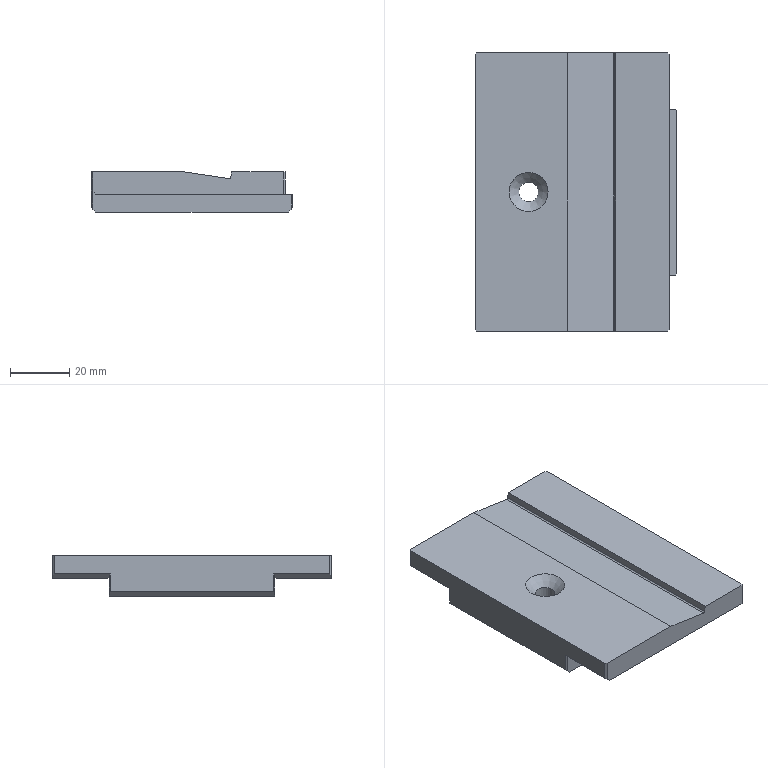Part | NX | 1 solid | 30 faces | box 68 x 94 x 13.65 mm | volume 67246 mm3 | plane 27 | cylinder 2 | cone 1 | commonest cylinder face diameters 1 x1 6.6 x1
STEP:
#1=CARTESIAN_POINT('',(-34.,27.5,1.5));
#2=VERTEX_POINT('',#1);
#3=CARTESIAN_POINT('',(-34.,-27.5,1.5));
#4=VERTEX_POINT('',#3);
#5=CARTESIAN_POINT('',(-34.,47.,1.5));
#6=DIRECTION('',(0.,-1.,0.));
#7=VECTOR('',#6,1000.);
#8=LINE('',#5,#7);
#9=EDGE_CURVE('',#2,#4,#8,.T.);
#10=ORIENTED_EDGE('',*,*,#9,.T.);
#11=CARTESIAN_POINT('',(-34.,-27.5,7.5));
#12=VERTEX_POINT('',#11);
#13=CARTESIAN_POINT('',(-34.,-27.5,13.65));
#14=DIRECTION('',(0.,0.,1.));
#15=VECTOR('',#14,1000.);
#16=LINE('',#13,#15);
#17=EDGE_CURVE('',#4,#12,#16,.T.);
#18=ORIENTED_EDGE('',*,*,#17,.T.);
#19=CARTESIAN_POINT('',(-34.,-46.5,7.5));
#20=VERTEX_POINT('',#19);
#21=CARTESIAN_POINT('',(-34.,47.,7.5));
#22=DIRECTION('',(0.,1.,0.));
#23=VECTOR('',#22,1000.);
#24=LINE('',#21,#23);
#25=EDGE_CURVE('',#12,#20,#24,.F.);
#26=ORIENTED_EDGE('',*,*,#25,.T.);
#27=CARTESIAN_POINT('',(-34.,-46.5,13.65));
#28=VERTEX_POINT('',#27);
#29=CARTESIAN_POINT('',(-34.,-46.5,13.65));
#30=DIRECTION('',(0.,0.,1.));
#31=VECTOR('',#30,1000.);
#32=LINE('',#29,#31);
#33=EDGE_CURVE('',#20,#28,#32,.T.);
#34=ORIENTED_EDGE('',*,*,#33,.T.);
#35=CARTESIAN_POINT('',(-34.,46.5,13.65));
#36=VERTEX_POINT('',#35);
#37=CARTESIAN_POINT('',(-34.,47.,13.65));
#38=DIRECTION('',(0.,-1.,0.));
#39=VECTOR('',#38,1000.);
#40=LINE('',#37,#39);
#41=EDGE_CURVE('',#36,#28,#40,.T.);
#42=ORIENTED_EDGE('',*,*,#41,.F.);
#43=CARTESIAN_POINT('',(-34.,46.5,7.5));
#44=VERTEX_POINT('',#43);
#45=CARTESIAN_POINT('',(-34.,46.5,13.65));
#46=DIRECTION('',(0.,0.,-1.));
#47=VECTOR('',#46,1000.);
#48=LINE('',#45,#47);
#49=EDGE_CURVE('',#36,#44,#48,.T.);
#50=ORIENTED_EDGE('',*,*,#49,.T.);
#51=CARTESIAN_POINT('',(-34.,27.5,7.5));
#52=VERTEX_POINT('',#51);
#53=CARTESIAN_POINT('',(-34.,47.,7.5));
#54=DIRECTION('',(0.,1.,0.));
#55=VECTOR('',#54,1000.);
#56=LINE('',#53,#55);
#57=EDGE_CURVE('',#44,#52,#56,.F.);
#58=ORIENTED_EDGE('',*,*,#57,.T.);
#59=CARTESIAN_POINT('',(-34.,27.5,1.5));
#60=DIRECTION('',(0.,0.,-1.));
#61=VECTOR('',#60,1000.);
#62=LINE('',#59,#61);
#63=EDGE_CURVE('',#52,#2,#62,.T.);
#64=ORIENTED_EDGE('',*,*,#63,.T.);
#65=EDGE_LOOP('',(#10,#18,#26,#34,#42,#50,#58,#64));
#66=FACE_BOUND('',#65,.T.);
#67=CARTESIAN_POINT('',(-34.,47.,13.65));
#68=DIRECTION('',(1.,0.,0.));
#69=DIRECTION('',(0.,0.,-1.));
#70=AXIS2_PLACEMENT_3D('',#67,#68,#69);
#71=PLANE('',#70);
#72=ADVANCED_FACE('',(#66),#71,.F.);
#73=ORIENTED_EDGE('',*,*,#41,.T.);
#74=CARTESIAN_POINT('',(-33.5,-47.,13.65));
#75=VERTEX_POINT('',#74);
#76=CARTESIAN_POINT('',(-48.25,-32.25,13.65));
#77=DIRECTION('',(-0.7071,0.7071,0.));
#78=VECTOR('',#77,1000.);
#79=LINE('',#76,#78);
#80=EDGE_CURVE('',#28,#75,#79,.F.);
#81=ORIENTED_EDGE('',*,*,#80,.T.);
#82=CARTESIAN_POINT('',(-3.,-47.,13.65));
#83=VERTEX_POINT('',#82);
#84=CARTESIAN_POINT('',(-34.,-47.,13.65));
#85=DIRECTION('',(1.,0.,0.));
#86=VECTOR('',#85,1000.);
#87=LINE('',#84,#86);
#88=EDGE_CURVE('',#75,#83,#87,.T.);
#89=ORIENTED_EDGE('',*,*,#88,.T.);
#90=CARTESIAN_POINT('',(-3.,47.,13.65));
#91=VERTEX_POINT('',#90);
#92=CARTESIAN_POINT('',(-3.,0.,13.65));
#93=DIRECTION('',(0.,1.,0.));
#94=VECTOR('',#93,1000.);
#95=LINE('',#92,#94);
#96=EDGE_CURVE('',#83,#91,#95,.T.);
#97=ORIENTED_EDGE('',*,*,#96,.T.);
#98=CARTESIAN_POINT('',(-33.5,47.,13.65));
#99=VERTEX_POINT('',#98);
#100=CARTESIAN_POINT('',(34.,47.,13.65));
#101=DIRECTION('',(-1.,0.,0.));
#102=VECTOR('',#101,1000.);
#103=LINE('',#100,#102);
#104=EDGE_CURVE('',#91,#99,#103,.T.);
#105=ORIENTED_EDGE('',*,*,#104,.T.);
#106=CARTESIAN_POINT('',(-48.25,32.25,13.65));
#107=DIRECTION('',(0.7071,0.7071,0.));
#108=VECTOR('',#107,1000.);
#109=LINE('',#106,#108);
#110=EDGE_CURVE('',#99,#36,#109,.F.);
#111=ORIENTED_EDGE('',*,*,#110,.T.);
#112=EDGE_LOOP('',(#73,#81,#89,#97,#105,#111));
#113=FACE_BOUND('',#112,.T.);
#114=CARTESIAN_POINT('',(-9.4,0.,13.65));
#115=VERTEX_POINT('',#114);
#116=CARTESIAN_POINT('',(-16.,0.,13.65));
#117=DIRECTION('',(0.,0.,1.));
#118=DIRECTION('',(1.,0.,0.));
#119=AXIS2_PLACEMENT_3D('',#116,#117,#118);
#120=CIRCLE('',#119,6.6);
#121=EDGE_CURVE('',#115,#115,#120,.F.);
#122=ORIENTED_EDGE('',*,*,#121,.T.);
#123=EDGE_LOOP('',(#122));
#124=FACE_BOUND('',#123,.T.);
#125=CARTESIAN_POINT('',(-16.,0.,13.65));
#126=DIRECTION('',(0.,0.,1.));
#127=DIRECTION('',(1.,0.,0.));
#128=AXIS2_PLACEMENT_3D('',#125,#126,#127);
#129=PLANE('',#128);
#130=ADVANCED_FACE('',(#113,#124),#129,.T.);
#131=CARTESIAN_POINT('',(-12.7,0.,0.));
#132=VERTEX_POINT('',#131);
#133=CARTESIAN_POINT('',(-16.,0.,0.));
#134=DIRECTION('',(0.,0.,1.));
#135=DIRECTION('',(1.,0.,0.));
#136=AXIS2_PLACEMENT_3D('',#133,#134,#135);
#137=CIRCLE('',#136,3.3);
#138=EDGE_CURVE('',#132,#132,#137,.T.);
#139=ORIENTED_EDGE('',*,*,#138,.T.);
#140=EDGE_LOOP('',(#139));
#141=FACE_BOUND('',#140,.T.);
#142=CARTESIAN_POINT('',(-32.5,28.,0.));
#143=VERTEX_POINT('',#142);
#144=CARTESIAN_POINT('',(32.5,28.,0.));
#145=VERTEX_POINT('',#144);
#146=CARTESIAN_POINT('',(-16.,28.,0.));
#147=DIRECTION('',(-1.,0.,0.));
#148=VECTOR('',#147,1000.);
#149=LINE('',#146,#148);
#150=EDGE_CURVE('',#143,#145,#149,.F.);
#151=ORIENTED_EDGE('',*,*,#150,.T.);
#152=CARTESIAN_POINT('',(32.5,-28.,0.));
#153=VERTEX_POINT('',#152);
#154=CARTESIAN_POINT('',(32.5,0.,0.));
#155=DIRECTION('',(0.,-1.,0.));
#156=VECTOR('',#155,1000.);
#157=LINE('',#154,#156);
#158=EDGE_CURVE('',#145,#153,#157,.T.);
#159=ORIENTED_EDGE('',*,*,#158,.T.);
#160=CARTESIAN_POINT('',(-32.5,-28.,0.));
#161=VERTEX_POINT('',#160);
#162=CARTESIAN_POINT('',(-16.,-28.,0.));
#163=DIRECTION('',(-1.,0.,0.));
#164=VECTOR('',#163,1000.);
#165=LINE('',#162,#164);
#166=EDGE_CURVE('',#161,#153,#165,.F.);
#167=ORIENTED_EDGE('',*,*,#166,.F.);
#168=CARTESIAN_POINT('',(-32.5,0.,0.));
#169=DIRECTION('',(0.,1.,0.));
#170=VECTOR('',#169,1000.);
#171=LINE('',#168,#170);
#172=EDGE_CURVE('',#161,#143,#171,.T.);
#173=ORIENTED_EDGE('',*,*,#172,.T.);
#174=EDGE_LOOP('',(#151,#159,#167,#173));
#175=FACE_BOUND('',#174,.T.);
#176=CARTESIAN_POINT('',(-16.,0.,0.));
#177=DIRECTION('',(0.,0.,1.));
#178=DIRECTION('',(1.,0.,0.));
#179=AXIS2_PLACEMENT_3D('',#176,#177,#178);
#180=PLANE('',#179);
#181=ADVANCED_FACE('',(#141,#175),#180,.F.);
#182=CARTESIAN_POINT('',(31.4,46.5,13.65));
#183=VERTEX_POINT('',#182);
#184=CARTESIAN_POINT('',(31.4,-46.5,13.65));
#185=VERTEX_POINT('',#184);
#186=CARTESIAN_POINT('',(31.4,0.,13.65));
#187=DIRECTION('',(0.,-1.,0.));
#188=VECTOR('',#187,1000.);
#189=LINE('',#186,#188);
#190=EDGE_CURVE('',#183,#185,#189,.T.);
#191=ORIENTED_EDGE('',*,*,#190,.T.);
#192=CARTESIAN_POINT('',(31.4,-46.5,6.));
#193=VERTEX_POINT('',#192);
#194=CARTESIAN_POINT('',(31.4,-46.5,6.));
#195=DIRECTION('',(0.,0.,-1.));
#196=VECTOR('',#195,1000.);
#197=LINE('',#194,#196);
#198=EDGE_CURVE('',#185,#193,#197,.T.);
#199=ORIENTED_EDGE('',*,*,#198,.T.);
#200=CARTESIAN_POINT('',(31.4,-28.,6.));
#201=VERTEX_POINT('',#200);
#202=CARTESIAN_POINT('',(31.4,0.,6.));
#203=DIRECTION('',(0.,1.,0.));
#204=VECTOR('',#203,1000.);
#205=LINE('',#202,#204);
#206=EDGE_CURVE('',#201,#193,#205,.F.);
#207=ORIENTED_EDGE('',*,*,#206,.F.);
#208=CARTESIAN_POINT('',(31.4,28.,6.));
#209=VERTEX_POINT('',#208);
#210=CARTESIAN_POINT('',(31.4,0.,6.));
#211=DIRECTION('',(0.,1.,0.));
#212=VECTOR('',#211,1000.);
#213=LINE('',#210,#212);
#214=EDGE_CURVE('',#209,#201,#213,.F.);
#215=ORIENTED_EDGE('',*,*,#214,.F.);
#216=CARTESIAN_POINT('',(31.4,46.5,6.));
#217=VERTEX_POINT('',#216);
#218=CARTESIAN_POINT('',(31.4,0.,6.));
#219=DIRECTION('',(0.,1.,0.));
#220=VECTOR('',#219,1000.);
#221=LINE('',#218,#220);
#222=EDGE_CURVE('',#217,#209,#221,.F.);
#223=ORIENTED_EDGE('',*,*,#222,.F.);
#224=CARTESIAN_POINT('',(31.4,46.5,13.65));
#225=DIRECTION('',(0.,0.,1.));
#226=VECTOR('',#225,1000.);
#227=LINE('',#224,#226);
#228=EDGE_CURVE('',#217,#183,#227,.T.);
#229=ORIENTED_EDGE('',*,*,#228,.T.);
#230=EDGE_LOOP('',(#191,#199,#207,#215,#223,#229));
#231=FACE_BOUND('',#230,.T.);
#232=CARTESIAN_POINT('',(31.4,0.,6.825));
#233=DIRECTION('',(1.,0.,0.));
#234=DIRECTION('',(0.,0.,-1.));
#235=AXIS2_PLACEMENT_3D('',#232,#233,#234);
#236=PLANE('',#235);
#237=ADVANCED_FACE('',(#231),#236,.T.);
#238=CARTESIAN_POINT('',(34.,27.5,6.));
#239=VERTEX_POINT('',#238);
#240=CARTESIAN_POINT('',(34.,-27.5,6.));
#241=VERTEX_POINT('',#240);
#242=CARTESIAN_POINT('',(34.,-47.,6.));
#243=DIRECTION('',(0.,-1.,0.));
#244=VECTOR('',#243,1000.);
#245=LINE('',#242,#244);
#246=EDGE_CURVE('',#239,#241,#245,.T.);
#247=ORIENTED_EDGE('',*,*,#246,.T.);
#248=CARTESIAN_POINT('',(34.,-27.5,1.5));
#249=VERTEX_POINT('',#248);
#250=CARTESIAN_POINT('',(34.,-27.5,13.65));
#251=DIRECTION('',(0.,0.,-1.));
#252=VECTOR('',#251,1000.);
#253=LINE('',#250,#252);
#254=EDGE_CURVE('',#241,#249,#253,.T.);
#255=ORIENTED_EDGE('',*,*,#254,.T.);
#256=CARTESIAN_POINT('',(34.,27.5,1.5));
#257=VERTEX_POINT('',#256);
#258=CARTESIAN_POINT('',(34.,-47.,1.5));
#259=DIRECTION('',(0.,1.,0.));
#260=VECTOR('',#259,1000.);
#261=LINE('',#258,#260);
#262=EDGE_CURVE('',#249,#257,#261,.T.);
#263=ORIENTED_EDGE('',*,*,#262,.T.);
#264=CARTESIAN_POINT('',(34.,27.5,6.));
#265=DIRECTION('',(0.,0.,1.));
#266=VECTOR('',#265,1000.);
#267=LINE('',#264,#266);
#268=EDGE_CURVE('',#257,#239,#267,.T.);
#269=ORIENTED_EDGE('',*,*,#268,.T.);
#270=EDGE_LOOP('',(#247,#255,#263,#269));
#271=FACE_BOUND('',#270,.T.);
#272=CARTESIAN_POINT('',(34.,-47.,13.65));
#273=DIRECTION('',(-1.,0.,0.));
#274=DIRECTION('',(0.,0.,1.));
#275=AXIS2_PLACEMENT_3D('',#272,#273,#274);
#276=PLANE('',#275);
#277=ADVANCED_FACE('',(#271),#276,.F.);
#278=CARTESIAN_POINT('',(33.5,-28.,6.));
#279=VERTEX_POINT('',#278);
#280=CARTESIAN_POINT('',(32.7,-28.,6.));
#281=DIRECTION('',(1.,0.,0.));
#282=VECTOR('',#281,1000.);
#283=LINE('',#280,#282);
#284=EDGE_CURVE('',#201,#279,#283,.T.);
#285=ORIENTED_EDGE('',*,*,#284,.T.);
#286=CARTESIAN_POINT('',(33.5,-28.,6.));
#287=DIRECTION('',(-0.7071,-0.7071,0.));
#288=VECTOR('',#287,1000.);
#289=LINE('',#286,#288);
#290=EDGE_CURVE('',#279,#241,#289,.F.);
#291=ORIENTED_EDGE('',*,*,#290,.T.);
#292=ORIENTED_EDGE('',*,*,#246,.F.);
#293=CARTESIAN_POINT('',(33.5,28.,6.));
#294=VERTEX_POINT('',#293);
#295=CARTESIAN_POINT('',(34.,27.5,6.));
#296=DIRECTION('',(-0.7071,0.7071,0.));
#297=VECTOR('',#296,1000.);
#298=LINE('',#295,#297);
#299=EDGE_CURVE('',#239,#294,#298,.T.);
#300=ORIENTED_EDGE('',*,*,#299,.T.);
#301=CARTESIAN_POINT('',(32.7,28.,6.));
#302=DIRECTION('',(1.,0.,0.));
#303=VECTOR('',#302,1000.);
#304=LINE('',#301,#303);
#305=EDGE_CURVE('',#209,#294,#304,.T.);
#306=ORIENTED_EDGE('',*,*,#305,.F.);
#307=ORIENTED_EDGE('',*,*,#214,.T.);
#308=EDGE_LOOP('',(#285,#291,#292,#300,#306,#307));
#309=FACE_BOUND('',#308,.T.);
#310=CARTESIAN_POINT('',(32.7,0.,6.));
#311=DIRECTION('',(0.,0.,-1.));
#312=DIRECTION('',(-1.,0.,0.));
#313=AXIS2_PLACEMENT_3D('',#310,#311,#312);
#314=PLANE('',#313);
#315=ADVANCED_FACE('',(#309),#314,.F.);
#316=ORIENTED_EDGE('',*,*,#96,.F.);
#317=CARTESIAN_POINT('',(12.531,-47.,11.329));
#318=VERTEX_POINT('',#317);
#319=CARTESIAN_POINT('',(-3.,-47.,13.65));
#320=DIRECTION('',(0.989,0.,-0.1478));
#321=VECTOR('',#320,1000.);
#322=LINE('',#319,#321);
#323=EDGE_CURVE('',#83,#318,#322,.T.);
#324=ORIENTED_EDGE('',*,*,#323,.T.);
#325=CARTESIAN_POINT('',(12.531,47.,11.329));
#326=VERTEX_POINT('',#325);
#327=CARTESIAN_POINT('',(12.531,47.,11.329));
#328=DIRECTION('',(0.,-1.,0.));
#329=VECTOR('',#328,1000.);
#330=LINE('',#327,#329);
#331=EDGE_CURVE('',#318,#326,#330,.F.);
#332=ORIENTED_EDGE('',*,*,#331,.T.);
#333=CARTESIAN_POINT('',(-3.,47.,13.65));
#334=DIRECTION('',(0.989,0.,-0.1478));
#335=VECTOR('',#334,1000.);
#336=LINE('',#333,#335);
#337=EDGE_CURVE('',#91,#326,#336,.T.);
#338=ORIENTED_EDGE('',*,*,#337,.F.);
#339=EDGE_LOOP('',(#316,#324,#332,#338));
#340=FACE_BOUND('',#339,.T.);
#341=CARTESIAN_POINT('',(-3.,47.,13.65));
#342=DIRECTION('',(-0.1478,0.,-0.989));
#343=DIRECTION('',(-0.989,0.,0.1478));
#344=AXIS2_PLACEMENT_3D('',#341,#342,#343);
#345=PLANE('',#344);
#346=ADVANCED_FACE('',(#340),#345,.F.);
#347=CARTESIAN_POINT('',(13.099,47.,11.75));
#348=VERTEX_POINT('',#347);
#349=CARTESIAN_POINT('',(13.099,-47.,11.75));
#350=VERTEX_POINT('',#349);
#351=CARTESIAN_POINT('',(13.099,0.,11.75));
#352=DIRECTION('',(0.,-1.,0.));
#353=VECTOR('',#352,1000.);
#354=LINE('',#351,#353);
#355=EDGE_CURVE('',#348,#350,#354,.T.);
#356=ORIENTED_EDGE('',*,*,#355,.T.);
#357=CARTESIAN_POINT('',(13.383,-47.,13.65));
#358=VERTEX_POINT('',#357);
#359=CARTESIAN_POINT('',(13.025,-47.,11.255));
#360=DIRECTION('',(-0.1478,0.,-0.989));
#361=VECTOR('',#360,1000.);
#362=LINE('',#359,#361);
#363=EDGE_CURVE('',#358,#350,#362,.T.);
#364=ORIENTED_EDGE('',*,*,#363,.F.);
#365=CARTESIAN_POINT('',(13.383,47.,13.65));
#366=VERTEX_POINT('',#365);
#367=CARTESIAN_POINT('',(13.383,0.,13.65));
#368=DIRECTION('',(0.,1.,0.));
#369=VECTOR('',#368,1000.);
#370=LINE('',#367,#369);
#371=EDGE_CURVE('',#358,#366,#370,.T.);
#372=ORIENTED_EDGE('',*,*,#371,.T.);
#373=CARTESIAN_POINT('',(13.834,47.,16.664));
#374=DIRECTION('',(-0.1478,0.,-0.989));
#375=VECTOR('',#374,1000.);
#376=LINE('',#373,#375);
#377=EDGE_CURVE('',#366,#348,#376,.T.);
#378=ORIENTED_EDGE('',*,*,#377,.T.);
#379=EDGE_LOOP('',(#356,#364,#372,#378));
#380=FACE_BOUND('',#379,.T.);
#381=CARTESIAN_POINT('',(13.025,0.,11.255));
#382=DIRECTION('',(-0.989,0.,0.1478));
#383=DIRECTION('',(0.1478,0.,0.989));
#384=AXIS2_PLACEMENT_3D('',#381,#382,#383);
#385=PLANE('',#384);
#386=ADVANCED_FACE('',(#380),#385,.T.);
#387=CARTESIAN_POINT('',(30.9,-47.,13.65));
#388=VERTEX_POINT('',#387);
#389=CARTESIAN_POINT('',(-34.,-47.,13.65));
#390=DIRECTION('',(-1.,0.,0.));
#391=VECTOR('',#390,1000.);
#392=LINE('',#389,#391);
#393=EDGE_CURVE('',#388,#358,#392,.T.);
#394=ORIENTED_EDGE('',*,*,#393,.F.);
#395=CARTESIAN_POINT('',(31.4,-46.5,13.65));
#396=DIRECTION('',(0.7071,0.7071,0.));
#397=VECTOR('',#396,1000.);
#398=LINE('',#395,#397);
#399=EDGE_CURVE('',#388,#185,#398,.T.);
#400=ORIENTED_EDGE('',*,*,#399,.T.);
#401=ORIENTED_EDGE('',*,*,#190,.F.);
#402=CARTESIAN_POINT('',(30.9,47.,13.65));
#403=VERTEX_POINT('',#402);
#404=CARTESIAN_POINT('',(31.4,46.5,13.65));
#405=DIRECTION('',(-0.7071,0.7071,0.));
#406=VECTOR('',#405,1000.);
#407=LINE('',#404,#406);
#408=EDGE_CURVE('',#183,#403,#407,.T.);
#409=ORIENTED_EDGE('',*,*,#408,.T.);
#410=CARTESIAN_POINT('',(34.,47.,13.65));
#411=DIRECTION('',(1.,0.,0.));
#412=VECTOR('',#411,1000.);
#413=LINE('',#410,#412);
#414=EDGE_CURVE('',#366,#403,#413,.T.);
#415=ORIENTED_EDGE('',*,*,#414,.F.);
#416=ORIENTED_EDGE('',*,*,#371,.F.);
#417=EDGE_LOOP('',(#394,#400,#401,#409,#415,#416));
#418=FACE_BOUND('',#417,.T.);
#419=CARTESIAN_POINT('',(0.,0.,13.65));
#420=DIRECTION('',(0.,0.,-1.));
#421=DIRECTION('',(-1.,0.,0.));
#422=AXIS2_PLACEMENT_3D('',#419,#420,#421);
#423=PLANE('',#422);
#424=ADVANCED_FACE('',(#418),#423,.F.);
#425=CARTESIAN_POINT('',(-33.5,-28.,1.));
#426=VERTEX_POINT('',#425);
#427=CARTESIAN_POINT('',(-34.,-28.,1.5));
#428=DIRECTION('',(-0.7071,0.,0.7071));
#429=VECTOR('',#428,1000.);
#430=LINE('',#427,#429);
#431=EDGE_CURVE('',#426,#161,#430,.F.);
#432=ORIENTED_EDGE('',*,*,#431,.F.);
#433=CARTESIAN_POINT('',(-58.833,-2.667,26.333));
#434=DIRECTION('',(-0.5774,0.5774,0.5774));
#435=VECTOR('',#434,1000.);
#436=LINE('',#433,#435);
#437=EDGE_CURVE('',#426,#4,#436,.T.);
#438=ORIENTED_EDGE('',*,*,#437,.T.);
#439=ORIENTED_EDGE('',*,*,#9,.F.);
#440=CARTESIAN_POINT('',(-33.5,28.,1.));
#441=VERTEX_POINT('',#440);
#442=CARTESIAN_POINT('',(-27.5,34.,-5.));
#443=DIRECTION('',(-0.5774,-0.5774,0.5774));
#444=VECTOR('',#443,1000.);
#445=LINE('',#442,#444);
#446=EDGE_CURVE('',#2,#441,#445,.F.);
#447=ORIENTED_EDGE('',*,*,#446,.T.);
#448=CARTESIAN_POINT('',(-34.,28.,1.5));
#449=DIRECTION('',(-0.7071,0.,0.7071));
#450=VECTOR('',#449,1000.);
#451=LINE('',#448,#450);
#452=EDGE_CURVE('',#143,#441,#451,.T.);
#453=ORIENTED_EDGE('',*,*,#452,.F.);
#454=ORIENTED_EDGE('',*,*,#172,.F.);
#455=EDGE_LOOP('',(#432,#438,#439,#447,#453,#454));
#456=FACE_BOUND('',#455,.T.);
#457=CARTESIAN_POINT('',(-34.,47.,1.5));
#458=DIRECTION('',(0.7071,0.,0.7071));
#459=DIRECTION('',(0.,-1.,0.));
#460=AXIS2_PLACEMENT_3D('',#457,#458,#459);
#461=PLANE('',#460);
#462=ADVANCED_FACE('',(#456),#461,.F.);
#463=ORIENTED_EDGE('',*,*,#331,.F.);
#464=CARTESIAN_POINT('',(12.605,-47.,11.823));
#465=DIRECTION('',(0.,1.,0.));
#466=DIRECTION('',(0.,0.,1.));
#467=AXIS2_PLACEMENT_3D('',#464,#465,#466);
#468=CIRCLE('',#467,0.5);
#469=EDGE_CURVE('',#350,#318,#468,.T.);
#470=ORIENTED_EDGE('',*,*,#469,.F.);
#471=ORIENTED_EDGE('',*,*,#355,.F.);
#472=CARTESIAN_POINT('',(12.605,47.,11.823));
#473=DIRECTION('',(0.,-1.,0.));
#474=DIRECTION('',(0.,0.,-1.));
#475=AXIS2_PLACEMENT_3D('',#472,#473,#474);
#476=CIRCLE('',#475,0.5);
#477=EDGE_CURVE('',#326,#348,#476,.T.);
#478=ORIENTED_EDGE('',*,*,#477,.F.);
#479=EDGE_LOOP('',(#463,#470,#471,#478));
#480=FACE_BOUND('',#479,.T.);
#481=CARTESIAN_POINT('',(12.605,0.,11.823));
#482=DIRECTION('',(0.,-1.,0.));
#483=DIRECTION('',(0.,0.,-1.));
#484=AXIS2_PLACEMENT_3D('',#481,#482,#483);
#485=CYLINDRICAL_SURFACE('',#484,0.5);
#486=ADVANCED_FACE('',(#480),#485,.F.);
#487=ORIENTED_EDGE('',*,*,#121,.F.);
#488=EDGE_LOOP('',(#487));
#489=FACE_BOUND('',#488,.T.);
#490=CARTESIAN_POINT('',(-12.7,0.,10.35));
#491=VERTEX_POINT('',#490);
#492=CARTESIAN_POINT('',(-16.,0.,10.35));
#493=DIRECTION('',(0.,0.,1.));
#494=DIRECTION('',(1.,0.,0.));
#495=AXIS2_PLACEMENT_3D('',#492,#493,#494);
#496=CIRCLE('',#495,3.3);
#497=EDGE_CURVE('',#491,#491,#496,.T.);
#498=ORIENTED_EDGE('',*,*,#497,.F.);
#499=EDGE_LOOP('',(#498));
#500=FACE_BOUND('',#499,.T.);
#501=CARTESIAN_POINT('',(-16.,0.,10.35));
#502=DIRECTION('',(0.,0.,1.));
#503=DIRECTION('',(1.,0.,0.));
#504=AXIS2_PLACEMENT_3D('',#501,#502,#503);
#505=CONICAL_SURFACE('',#504,3.3,0.7854);
#506=ADVANCED_FACE('',(#489,#500),#505,.F.);
#507=ORIENTED_EDGE('',*,*,#497,.T.);
#508=EDGE_LOOP('',(#507));
#509=FACE_BOUND('',#508,.T.);
#510=ORIENTED_EDGE('',*,*,#138,.F.);
#511=EDGE_LOOP('',(#510));
#512=FACE_BOUND('',#511,.T.);
#513=CARTESIAN_POINT('',(-16.,0.,13.65));
#514=DIRECTION('',(0.,0.,-1.));
#515=DIRECTION('',(-1.,0.,0.));
#516=AXIS2_PLACEMENT_3D('',#513,#514,#515);
#517=CYLINDRICAL_SURFACE('',#516,3.3);
#518=ADVANCED_FACE('',(#509,#512),#517,.F.);
#519=ORIENTED_EDGE('',*,*,#305,.T.);
#520=CARTESIAN_POINT('',(33.5,28.,1.));
#521=VERTEX_POINT('',#520);
#522=CARTESIAN_POINT('',(33.5,28.,1.5));
#523=DIRECTION('',(0.,0.,-1.));
#524=VECTOR('',#523,1000.);
#525=LINE('',#522,#524);
#526=EDGE_CURVE('',#294,#521,#525,.T.);
#527=ORIENTED_EDGE('',*,*,#526,.T.);
#528=CARTESIAN_POINT('',(19.663,28.,-12.838));
#529=DIRECTION('',(0.7071,0.,0.7071));
#530=VECTOR('',#529,1000.);
#531=LINE('',#528,#530);
#532=EDGE_CURVE('',#521,#145,#531,.F.);
#533=ORIENTED_EDGE('',*,*,#532,.T.);
#534=ORIENTED_EDGE('',*,*,#150,.F.);
#535=ORIENTED_EDGE('',*,*,#452,.T.);
#536=CARTESIAN_POINT('',(-33.5,28.,7.));
#537=VERTEX_POINT('',#536);
#538=CARTESIAN_POINT('',(-33.5,28.,7.5));
#539=DIRECTION('',(0.,0.,1.));
#540=VECTOR('',#539,1000.);
#541=LINE('',#538,#540);
#542=EDGE_CURVE('',#441,#537,#541,.T.);
#543=ORIENTED_EDGE('',*,*,#542,.T.);
#544=CARTESIAN_POINT('',(-32.5,28.,6.));
#545=VERTEX_POINT('',#544);
#546=CARTESIAN_POINT('',(-34.,28.,7.5));
#547=DIRECTION('',(-0.7071,0.,0.7071));
#548=VECTOR('',#547,1000.);
#549=LINE('',#546,#548);
#550=EDGE_CURVE('',#537,#545,#549,.F.);
#551=ORIENTED_EDGE('',*,*,#550,.T.);
#552=CARTESIAN_POINT('',(-16.,28.,6.));
#553=DIRECTION('',(-1.,0.,0.));
#554=VECTOR('',#553,1000.);
#555=LINE('',#552,#554);
#556=EDGE_CURVE('',#209,#545,#555,.T.);
#557=ORIENTED_EDGE('',*,*,#556,.F.);
#558=EDGE_LOOP('',(#519,#527,#533,#534,#535,#543,#551,#557));
#559=FACE_BOUND('',#558,.T.);
#560=CARTESIAN_POINT('',(0.,28.,6.825));
#561=DIRECTION('',(0.,1.,0.));
#562=DIRECTION('',(0.,0.,1.));
#563=AXIS2_PLACEMENT_3D('',#560,#561,#562);
#564=PLANE('',#563);
#565=ADVANCED_FACE('',(#559),#564,.T.);
#566=CARTESIAN_POINT('',(33.5,-28.,1.));
#567=VERTEX_POINT('',#566);
#568=CARTESIAN_POINT('',(34.,-28.,1.5));
#569=DIRECTION('',(-0.7071,0.,-0.7071));
#570=VECTOR('',#569,1000.);
#571=LINE('',#568,#570);
#572=EDGE_CURVE('',#153,#567,#571,.F.);
#573=ORIENTED_EDGE('',*,*,#572,.T.);
#574=CARTESIAN_POINT('',(33.5,-28.,6.825));
#575=DIRECTION('',(0.,0.,1.));
#576=VECTOR('',#575,1000.);
#577=LINE('',#574,#576);
#578=EDGE_CURVE('',#567,#279,#577,.T.);
#579=ORIENTED_EDGE('',*,*,#578,.T.);
#580=ORIENTED_EDGE('',*,*,#284,.F.);
#581=CARTESIAN_POINT('',(-32.5,-28.,6.));
#582=VERTEX_POINT('',#581);
#583=CARTESIAN_POINT('',(-16.,-28.,6.));
#584=DIRECTION('',(-1.,0.,0.));
#585=VECTOR('',#584,1000.);
#586=LINE('',#583,#585);
#587=EDGE_CURVE('',#201,#582,#586,.T.);
#588=ORIENTED_EDGE('',*,*,#587,.T.);
#589=CARTESIAN_POINT('',(-33.5,-28.,7.));
#590=VERTEX_POINT('',#589);
#591=CARTESIAN_POINT('',(-16.663,-28.,-9.838));
#592=DIRECTION('',(0.7071,0.,-0.7071));
#593=VECTOR('',#592,1000.);
#594=LINE('',#591,#593);
#595=EDGE_CURVE('',#582,#590,#594,.F.);
#596=ORIENTED_EDGE('',*,*,#595,.T.);
#597=CARTESIAN_POINT('',(-33.5,-28.,6.825));
#598=DIRECTION('',(0.,0.,-1.));
#599=VECTOR('',#598,1000.);
#600=LINE('',#597,#599);
#601=EDGE_CURVE('',#590,#426,#600,.T.);
#602=ORIENTED_EDGE('',*,*,#601,.T.);
#603=ORIENTED_EDGE('',*,*,#431,.T.);
#604=ORIENTED_EDGE('',*,*,#166,.T.);
#605=EDGE_LOOP('',(#573,#579,#580,#588,#596,#602,#603,#604));
#606=FACE_BOUND('',#605,.T.);
#607=CARTESIAN_POINT('',(0.,-28.,6.825));
#608=DIRECTION('',(0.,1.,0.));
#609=DIRECTION('',(0.,0.,1.));
#610=AXIS2_PLACEMENT_3D('',#607,#608,#609);
#611=PLANE('',#610);
#612=ADVANCED_FACE('',(#606),#611,.F.);
#613=ORIENTED_EDGE('',*,*,#414,.T.);
#614=CARTESIAN_POINT('',(30.9,47.,6.));
#615=VERTEX_POINT('',#614);
#616=CARTESIAN_POINT('',(30.9,47.,6.));
#617=DIRECTION('',(0.,0.,-1.));
#618=VECTOR('',#617,1000.);
#619=LINE('',#616,#618);
#620=EDGE_CURVE('',#403,#615,#619,.T.);
#621=ORIENTED_EDGE('',*,*,#620,.T.);
#622=CARTESIAN_POINT('',(-32.5,47.,6.));
#623=VERTEX_POINT('',#622);
#624=CARTESIAN_POINT('',(34.,47.,6.));
#625=DIRECTION('',(-1.,0.,0.));
#626=VECTOR('',#625,1000.);
#627=LINE('',#624,#626);
#628=EDGE_CURVE('',#615,#623,#627,.T.);
#629=ORIENTED_EDGE('',*,*,#628,.T.);
#630=CARTESIAN_POINT('',(-33.5,47.,7.));
#631=VERTEX_POINT('',#630);
#632=CARTESIAN_POINT('',(-34.,47.,7.5));
#633=DIRECTION('',(0.7071,0.,-0.7071));
#634=VECTOR('',#633,1000.);
#635=LINE('',#632,#634);
#636=EDGE_CURVE('',#623,#631,#635,.F.);
#637=ORIENTED_EDGE('',*,*,#636,.T.);
#638=CARTESIAN_POINT('',(-33.5,47.,13.65));
#639=DIRECTION('',(0.,0.,1.));
#640=VECTOR('',#639,1000.);
#641=LINE('',#638,#640);
#642=EDGE_CURVE('',#631,#99,#641,.T.);
#643=ORIENTED_EDGE('',*,*,#642,.T.);
#644=ORIENTED_EDGE('',*,*,#104,.F.);
#645=ORIENTED_EDGE('',*,*,#337,.T.);
#646=ORIENTED_EDGE('',*,*,#477,.T.);
#647=ORIENTED_EDGE('',*,*,#377,.F.);
#648=EDGE_LOOP('',(#613,#621,#629,#637,#643,#644,#645,#646,#647));
#649=FACE_BOUND('',#648,.T.);
#650=CARTESIAN_POINT('',(34.,47.,13.65));
#651=DIRECTION('',(0.,-1.,0.));
#652=DIRECTION('',(0.,0.,-1.));
#653=AXIS2_PLACEMENT_3D('',#650,#651,#652);
#654=PLANE('',#653);
#655=ADVANCED_FACE('',(#649),#654,.F.);
#656=ORIENTED_EDGE('',*,*,#57,.F.);
#657=CARTESIAN_POINT('',(-33.833,46.667,7.333));
#658=DIRECTION('',(0.5774,0.5774,-0.5774));
#659=VECTOR('',#658,1000.);
#660=LINE('',#657,#659);
#661=EDGE_CURVE('',#44,#631,#660,.T.);
#662=ORIENTED_EDGE('',*,*,#661,.T.);
#663=ORIENTED_EDGE('',*,*,#636,.F.);
#664=CARTESIAN_POINT('',(-32.5,47.,6.));
#665=DIRECTION('',(0.,-1.,0.));
#666=VECTOR('',#665,1000.);
#667=LINE('',#664,#666);
#668=EDGE_CURVE('',#545,#623,#667,.F.);
#669=ORIENTED_EDGE('',*,*,#668,.F.);
#670=ORIENTED_EDGE('',*,*,#550,.F.);
#671=CARTESIAN_POINT('',(-36.05,25.45,9.55));
#672=DIRECTION('',(0.5774,0.5774,-0.5774));
#673=VECTOR('',#672,1000.);
#674=LINE('',#671,#673);
#675=EDGE_CURVE('',#537,#52,#674,.F.);
#676=ORIENTED_EDGE('',*,*,#675,.T.);
#677=EDGE_LOOP('',(#656,#662,#663,#669,#670,#676));
#678=FACE_BOUND('',#677,.T.);
#679=CARTESIAN_POINT('',(-34.,47.,7.5));
#680=DIRECTION('',(0.7071,0.,0.7071));
#681=DIRECTION('',(0.7071,0.,-0.7071));
#682=AXIS2_PLACEMENT_3D('',#679,#680,#681);
#683=PLANE('',#682);
#684=ADVANCED_FACE('',(#678),#683,.F.);
#685=ORIENTED_EDGE('',*,*,#628,.F.);
#686=CARTESIAN_POINT('',(31.4,46.5,6.));
#687=DIRECTION('',(0.7071,-0.7071,0.));
#688=VECTOR('',#687,1000.);
#689=LINE('',#686,#688);
#690=EDGE_CURVE('',#615,#217,#689,.T.);
#691=ORIENTED_EDGE('',*,*,#690,.T.);
#692=ORIENTED_EDGE('',*,*,#222,.T.);
#693=ORIENTED_EDGE('',*,*,#556,.T.);
#694=ORIENTED_EDGE('',*,*,#668,.T.);
#695=EDGE_LOOP('',(#685,#691,#692,#693,#694));
#696=FACE_BOUND('',#695,.T.);
#697=CARTESIAN_POINT('',(-16.,0.,6.));
#698=DIRECTION('',(0.,0.,1.));
#699=DIRECTION('',(1.,0.,0.));
#700=AXIS2_PLACEMENT_3D('',#697,#698,#699);
#701=PLANE('',#700);
#702=ADVANCED_FACE('',(#696),#701,.F.);
#703=ORIENTED_EDGE('',*,*,#88,.F.);
#704=CARTESIAN_POINT('',(-33.5,-47.,7.));
#705=VERTEX_POINT('',#704);
#706=CARTESIAN_POINT('',(-33.5,-47.,13.65));
#707=DIRECTION('',(0.,0.,-1.));
#708=VECTOR('',#707,1000.);
#709=LINE('',#706,#708);
#710=EDGE_CURVE('',#75,#705,#709,.T.);
#711=ORIENTED_EDGE('',*,*,#710,.T.);
#712=CARTESIAN_POINT('',(-32.5,-47.,6.));
#713=VERTEX_POINT('',#712);
#714=CARTESIAN_POINT('',(-34.,-47.,7.5));
#715=DIRECTION('',(-0.7071,0.,0.7071));
#716=VECTOR('',#715,1000.);
#717=LINE('',#714,#716);
#718=EDGE_CURVE('',#705,#713,#717,.F.);
#719=ORIENTED_EDGE('',*,*,#718,.T.);
#720=CARTESIAN_POINT('',(30.9,-47.,6.));
#721=VERTEX_POINT('',#720);
#722=CARTESIAN_POINT('',(-34.,-47.,6.));
#723=DIRECTION('',(1.,0.,0.));
#724=VECTOR('',#723,1000.);
#725=LINE('',#722,#724);
#726=EDGE_CURVE('',#713,#721,#725,.T.);
#727=ORIENTED_EDGE('',*,*,#726,.T.);
#728=CARTESIAN_POINT('',(30.9,-47.,13.65));
#729=DIRECTION('',(0.,0.,1.));
#730=VECTOR('',#729,1000.);
#731=LINE('',#728,#730);
#732=EDGE_CURVE('',#721,#388,#731,.T.);
#733=ORIENTED_EDGE('',*,*,#732,.T.);
#734=ORIENTED_EDGE('',*,*,#393,.T.);
#735=ORIENTED_EDGE('',*,*,#363,.T.);
#736=ORIENTED_EDGE('',*,*,#469,.T.);
#737=ORIENTED_EDGE('',*,*,#323,.F.);
#738=EDGE_LOOP('',(#703,#711,#719,#727,#733,#734,#735,#736,#737));
#739=FACE_BOUND('',#738,.T.);
#740=CARTESIAN_POINT('',(-34.,-47.,13.65));
#741=DIRECTION('',(0.,1.,0.));
#742=DIRECTION('',(0.,0.,1.));
#743=AXIS2_PLACEMENT_3D('',#740,#741,#742);
#744=PLANE('',#743);
#745=ADVANCED_FACE('',(#739),#744,.F.);
#746=ORIENTED_EDGE('',*,*,#718,.F.);
#747=CARTESIAN_POINT('',(-65.167,-15.333,38.667));
#748=DIRECTION('',(-0.5774,0.5774,0.5774));
#749=VECTOR('',#748,1000.);
#750=LINE('',#747,#749);
#751=EDGE_CURVE('',#705,#20,#750,.T.);
#752=ORIENTED_EDGE('',*,*,#751,.T.);
#753=ORIENTED_EDGE('',*,*,#25,.F.);
#754=CARTESIAN_POINT('',(-33.442,-28.058,6.942));
#755=DIRECTION('',(0.5774,-0.5774,-0.5774));
#756=VECTOR('',#755,1000.);
#757=LINE('',#754,#756);
#758=EDGE_CURVE('',#12,#590,#757,.T.);
#759=ORIENTED_EDGE('',*,*,#758,.T.);
#760=ORIENTED_EDGE('',*,*,#595,.F.);
#761=CARTESIAN_POINT('',(-32.5,47.,6.));
#762=DIRECTION('',(0.,-1.,0.));
#763=VECTOR('',#762,1000.);
#764=LINE('',#761,#763);
#765=EDGE_CURVE('',#713,#582,#764,.F.);
#766=ORIENTED_EDGE('',*,*,#765,.F.);
#767=EDGE_LOOP('',(#746,#752,#753,#759,#760,#766));
#768=FACE_BOUND('',#767,.T.);
#769=CARTESIAN_POINT('',(-34.,47.,7.5));
#770=DIRECTION('',(0.7071,0.,0.7071));
#771=DIRECTION('',(0.7071,0.,-0.7071));
#772=AXIS2_PLACEMENT_3D('',#769,#770,#771);
#773=PLANE('',#772);
#774=ADVANCED_FACE('',(#768),#773,.F.);
#775=ORIENTED_EDGE('',*,*,#206,.T.);
#776=CARTESIAN_POINT('',(31.4,-46.5,6.));
#777=DIRECTION('',(-0.7071,-0.7071,0.));
#778=VECTOR('',#777,1000.);
#779=LINE('',#776,#778);
#780=EDGE_CURVE('',#193,#721,#779,.T.);
#781=ORIENTED_EDGE('',*,*,#780,.T.);
#782=ORIENTED_EDGE('',*,*,#726,.F.);
#783=ORIENTED_EDGE('',*,*,#765,.T.);
#784=ORIENTED_EDGE('',*,*,#587,.F.);
#785=EDGE_LOOP('',(#775,#781,#782,#783,#784));
#786=FACE_BOUND('',#785,.T.);
#787=CARTESIAN_POINT('',(-16.,0.,6.));
#788=DIRECTION('',(0.,0.,1.));
#789=DIRECTION('',(1.,0.,0.));
#790=AXIS2_PLACEMENT_3D('',#787,#788,#789);
#791=PLANE('',#790);
#792=ADVANCED_FACE('',(#786),#791,.F.);
#793=ORIENTED_EDGE('',*,*,#262,.F.);
#794=CARTESIAN_POINT('',(27.5,-34.,-5.));
#795=DIRECTION('',(-0.5774,-0.5774,-0.5774));
#796=VECTOR('',#795,1000.);
#797=LINE('',#794,#796);
#798=EDGE_CURVE('',#249,#567,#797,.T.);
#799=ORIENTED_EDGE('',*,*,#798,.T.);
#800=ORIENTED_EDGE('',*,*,#572,.F.);
#801=ORIENTED_EDGE('',*,*,#158,.F.);
#802=ORIENTED_EDGE('',*,*,#532,.F.);
#803=CARTESIAN_POINT('',(58.833,2.667,26.333));
#804=DIRECTION('',(-0.5774,0.5774,-0.5774));
#805=VECTOR('',#804,1000.);
#806=LINE('',#803,#805);
#807=EDGE_CURVE('',#521,#257,#806,.F.);
#808=ORIENTED_EDGE('',*,*,#807,.T.);
#809=EDGE_LOOP('',(#793,#799,#800,#801,#802,#808));
#810=FACE_BOUND('',#809,.T.);
#811=CARTESIAN_POINT('',(34.,-47.,1.5));
#812=DIRECTION('',(-0.7071,0.,0.7071));
#813=DIRECTION('',(0.,1.,0.));
#814=AXIS2_PLACEMENT_3D('',#811,#812,#813);
#815=PLANE('',#814);
#816=ADVANCED_FACE('',(#810),#815,.F.);
#817=ORIENTED_EDGE('',*,*,#80,.F.);
#818=ORIENTED_EDGE('',*,*,#33,.F.);
#819=ORIENTED_EDGE('',*,*,#751,.F.);
#820=ORIENTED_EDGE('',*,*,#710,.F.);
#821=EDGE_LOOP('',(#817,#818,#819,#820));
#822=FACE_BOUND('',#821,.T.);
#823=CARTESIAN_POINT('',(-33.5,-47.,13.65));
#824=DIRECTION('',(0.7071,0.7071,0.));
#825=DIRECTION('',(0.,0.,-1.));
#826=AXIS2_PLACEMENT_3D('',#823,#824,#825);
#827=PLANE('',#826);
#828=ADVANCED_FACE('',(#822),#827,.F.);
#829=ORIENTED_EDGE('',*,*,#399,.F.);
#830=ORIENTED_EDGE('',*,*,#732,.F.);
#831=ORIENTED_EDGE('',*,*,#780,.F.);
#832=ORIENTED_EDGE('',*,*,#198,.F.);
#833=EDGE_LOOP('',(#829,#830,#831,#832));
#834=FACE_BOUND('',#833,.T.);
#835=CARTESIAN_POINT('',(31.4,-46.5,6.825));
#836=DIRECTION('',(0.7071,-0.7071,0.));
#837=DIRECTION('',(0.,0.,1.));
#838=AXIS2_PLACEMENT_3D('',#835,#836,#837);
#839=PLANE('',#838);
#840=ADVANCED_FACE('',(#834),#839,.T.);
#841=ORIENTED_EDGE('',*,*,#690,.F.);
#842=ORIENTED_EDGE('',*,*,#620,.F.);
#843=ORIENTED_EDGE('',*,*,#408,.F.);
#844=ORIENTED_EDGE('',*,*,#228,.F.);
#845=EDGE_LOOP('',(#841,#842,#843,#844));
#846=FACE_BOUND('',#845,.T.);
#847=CARTESIAN_POINT('',(31.4,46.5,6.825));
#848=DIRECTION('',(0.7071,0.7071,0.));
#849=DIRECTION('',(0.,0.,-1.));
#850=AXIS2_PLACEMENT_3D('',#847,#848,#849);
#851=PLANE('',#850);
#852=ADVANCED_FACE('',(#846),#851,.T.);
#853=ORIENTED_EDGE('',*,*,#110,.F.);
#854=ORIENTED_EDGE('',*,*,#642,.F.);
#855=ORIENTED_EDGE('',*,*,#661,.F.);
#856=ORIENTED_EDGE('',*,*,#49,.F.);
#857=EDGE_LOOP('',(#853,#854,#855,#856));
#858=FACE_BOUND('',#857,.T.);
#859=CARTESIAN_POINT('',(-34.,46.5,13.65));
#860=DIRECTION('',(0.7071,-0.7071,0.));
#861=DIRECTION('',(0.,0.,-1.));
#862=AXIS2_PLACEMENT_3D('',#859,#860,#861);
#863=PLANE('',#862);
#864=ADVANCED_FACE('',(#858),#863,.F.);
#865=ORIENTED_EDGE('',*,*,#798,.F.);
#866=ORIENTED_EDGE('',*,*,#254,.F.);
#867=ORIENTED_EDGE('',*,*,#290,.F.);
#868=ORIENTED_EDGE('',*,*,#578,.F.);
#869=EDGE_LOOP('',(#865,#866,#867,#868));
#870=FACE_BOUND('',#869,.T.);
#871=CARTESIAN_POINT('',(33.5,-28.,6.825));
#872=DIRECTION('',(-0.7071,0.7071,0.));
#873=DIRECTION('',(0.,0.,1.));
#874=AXIS2_PLACEMENT_3D('',#871,#872,#873);
#875=PLANE('',#874);
#876=ADVANCED_FACE('',(#870),#875,.F.);
#877=ORIENTED_EDGE('',*,*,#807,.F.);
#878=ORIENTED_EDGE('',*,*,#526,.F.);
#879=ORIENTED_EDGE('',*,*,#299,.F.);
#880=ORIENTED_EDGE('',*,*,#268,.F.);
#881=EDGE_LOOP('',(#877,#878,#879,#880));
#882=FACE_BOUND('',#881,.T.);
#883=CARTESIAN_POINT('',(34.,27.5,13.65));
#884=DIRECTION('',(0.7071,0.7071,0.));
#885=DIRECTION('',(0.,0.,-1.));
#886=AXIS2_PLACEMENT_3D('',#883,#884,#885);
#887=PLANE('',#886);
#888=ADVANCED_FACE('',(#882),#887,.T.);
#889=ORIENTED_EDGE('',*,*,#758,.F.);
#890=ORIENTED_EDGE('',*,*,#17,.F.);
#891=ORIENTED_EDGE('',*,*,#437,.F.);
#892=ORIENTED_EDGE('',*,*,#601,.F.);
#893=EDGE_LOOP('',(#889,#890,#891,#892));
#894=FACE_BOUND('',#893,.T.);
#895=CARTESIAN_POINT('',(-33.5,-28.,6.825));
#896=DIRECTION('',(0.7071,0.7071,0.));
#897=DIRECTION('',(0.,0.,-1.));
#898=AXIS2_PLACEMENT_3D('',#895,#896,#897);
#899=PLANE('',#898);
#900=ADVANCED_FACE('',(#894),#899,.F.);
#901=ORIENTED_EDGE('',*,*,#675,.F.);
#902=ORIENTED_EDGE('',*,*,#542,.F.);
#903=ORIENTED_EDGE('',*,*,#446,.F.);
#904=ORIENTED_EDGE('',*,*,#63,.F.);
#905=EDGE_LOOP('',(#901,#902,#903,#904));
#906=FACE_BOUND('',#905,.T.);
#907=CARTESIAN_POINT('',(-34.,27.5,13.65));
#908=DIRECTION('',(-0.7071,0.7071,0.));
#909=DIRECTION('',(0.,0.,1.));
#910=AXIS2_PLACEMENT_3D('',#907,#908,#909);
#911=PLANE('',#910);
#912=ADVANCED_FACE('',(#906),#911,.T.);
#913=CLOSED_SHELL('',(#72,#130,#181,#237,#277,#315,#346,#386,#424,#462,#486,#506,#518,#565,#612,#655,#684,#702,#745,#774,#792,#816,#828,#840,#852,#864,#876,#888,#900,#912));
#914=MANIFOLD_SOLID_BREP('',#913);
#915=(LENGTH_UNIT()NAMED_UNIT(*)SI_UNIT(.MILLI.,.METRE.));
#916=UNCERTAINTY_MEASURE_WITH_UNIT(LENGTH_MEASURE(0.00001),#915,'','');
#917=(NAMED_UNIT(*)PLANE_ANGLE_UNIT()SI_UNIT($,.RADIAN.));
#918=(NAMED_UNIT(*)SI_UNIT($,.STERADIAN.)SOLID_ANGLE_UNIT());
#919=(GEOMETRIC_REPRESENTATION_CONTEXT(3)GLOBAL_UNCERTAINTY_ASSIGNED_CONTEXT((#916))GLOBAL_UNIT_ASSIGNED_CONTEXT((#915,#917,#918))REPRESENTATION_CONTEXT('',''));
#920=ADVANCED_BREP_SHAPE_REPRESENTATION('',(#914),#919);